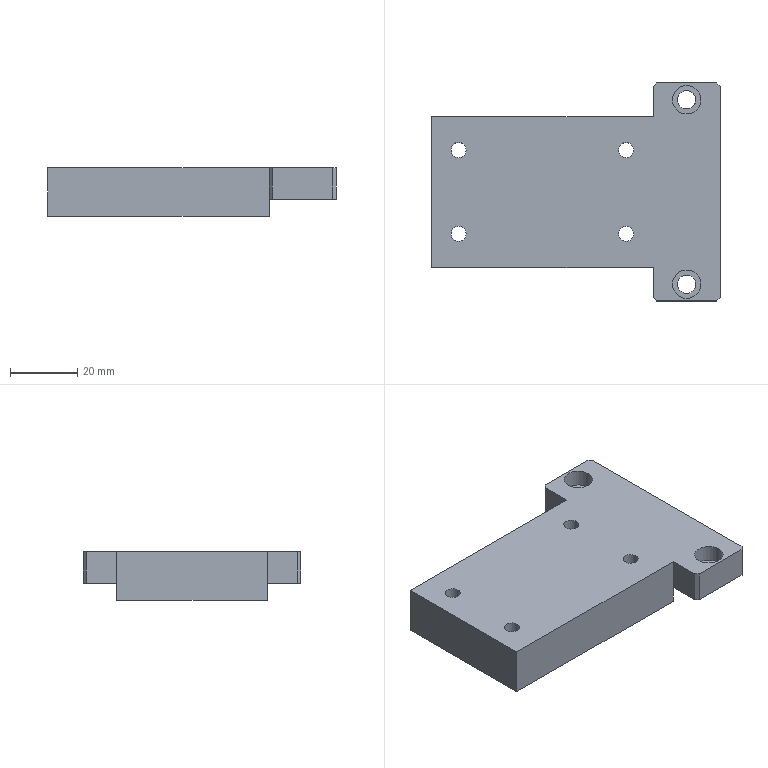Part | STEP file | Tube feed_id858_x_t | 1 solid | 34 faces | box 86 x 65 x 14.5 mm | volume 52880 mm3 | plane 22 | cylinder 12 | commonest cylinder face diameters 4.5 x4 8 x4 5.5 x2 8.5 x2